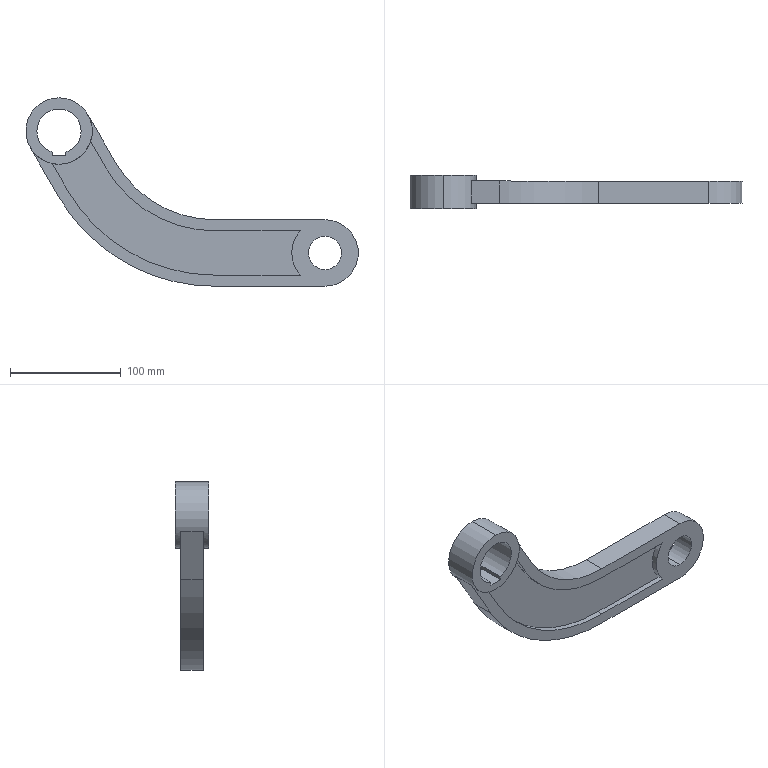Part | SolidWorks | features ICE 4, Extrusion 1 | 1 solid | 35 faces | box 300 x 30 x 170 mm | volume 285435 mm3 | plane 21 | cylinder 14 | commonest cylinder face diameters 60 x5 30 x2 226.795 x2 306.795 x2 40 x1 206.795 x1
STEP:
#1=CARTESIAN_POINT('',(240.,10.,-125.));
#2=VERTEX_POINT('',#1);
#3=CARTESIAN_POINT('',(240.,10.,-95.));
#4=VERTEX_POINT('',#3);
#5=CARTESIAN_POINT('',(240.,10.,-110.));
#6=DIRECTION('',(0.,1.,0.));
#7=DIRECTION('',(0.,0.,1.));
#8=AXIS2_PLACEMENT_3D('',#5,#6,#7);
#9=CIRCLE('',#8,15.);
#10=EDGE_CURVE('',#2,#4,#9,.T.);
#11=ORIENTED_EDGE('',*,*,#10,.T.);
#12=CARTESIAN_POINT('',(240.,-10.,-95.));
#13=VERTEX_POINT('',#12);
#14=CARTESIAN_POINT('',(240.,10.,-95.));
#15=DIRECTION('',(0.,-1.,0.));
#16=VECTOR('',#15,1000.);
#17=LINE('',#14,#16);
#18=EDGE_CURVE('',#4,#13,#17,.T.);
#19=ORIENTED_EDGE('',*,*,#18,.T.);
#20=CARTESIAN_POINT('',(240.,-10.,-125.));
#21=VERTEX_POINT('',#20);
#22=CARTESIAN_POINT('',(240.,-10.,-110.));
#23=DIRECTION('',(0.,1.,0.));
#24=DIRECTION('',(0.,0.,1.));
#25=AXIS2_PLACEMENT_3D('',#22,#23,#24);
#26=CIRCLE('',#25,15.);
#27=EDGE_CURVE('',#21,#13,#26,.T.);
#28=ORIENTED_EDGE('',*,*,#27,.F.);
#29=CARTESIAN_POINT('',(240.,10.,-125.));
#30=DIRECTION('',(0.,-1.,0.));
#31=VECTOR('',#30,1000.);
#32=LINE('',#29,#31);
#33=EDGE_CURVE('',#2,#21,#32,.T.);
#34=ORIENTED_EDGE('',*,*,#33,.F.);
#35=EDGE_LOOP('',(#11,#19,#28,#34));
#36=FACE_OUTER_BOUND('',#35,.T.);
#37=CARTESIAN_POINT('',(240.,10.,-110.));
#38=DIRECTION('',(0.,-1.,0.));
#39=DIRECTION('',(0.,0.,-1.));
#40=AXIS2_PLACEMENT_3D('',#37,#38,#39);
#41=CYLINDRICAL_SURFACE('',#40,15.);
#42=ADVANCED_FACE('',(#36),#41,.F.);
#43=CARTESIAN_POINT('',(0.,15.,30.));
#44=VERTEX_POINT('',#43);
#45=CARTESIAN_POINT('',(0.,15.,-30.));
#46=VERTEX_POINT('',#45);
#47=CARTESIAN_POINT('',(0.,15.,0.));
#48=DIRECTION('',(0.,1.,0.));
#49=DIRECTION('',(0.,0.,1.));
#50=AXIS2_PLACEMENT_3D('',#47,#48,#49);
#51=CIRCLE('',#50,30.);
#52=EDGE_CURVE('',#44,#46,#51,.T.);
#53=ORIENTED_EDGE('',*,*,#52,.F.);
#54=CARTESIAN_POINT('',(0.,-15.,30.));
#55=VERTEX_POINT('',#54);
#56=CARTESIAN_POINT('',(0.,15.,30.));
#57=DIRECTION('',(0.,-1.,0.));
#58=VECTOR('',#57,1000.);
#59=LINE('',#56,#58);
#60=EDGE_CURVE('',#44,#55,#59,.T.);
#61=ORIENTED_EDGE('',*,*,#60,.T.);
#62=CARTESIAN_POINT('',(0.,-15.,-30.));
#63=VERTEX_POINT('',#62);
#64=CARTESIAN_POINT('',(0.,-15.,0.));
#65=DIRECTION('',(0.,1.,0.));
#66=DIRECTION('',(0.,0.,1.));
#67=AXIS2_PLACEMENT_3D('',#64,#65,#66);
#68=CIRCLE('',#67,30.);
#69=EDGE_CURVE('',#55,#63,#68,.T.);
#70=ORIENTED_EDGE('',*,*,#69,.T.);
#71=CARTESIAN_POINT('',(0.,-5.,-30.));
#72=VERTEX_POINT('',#71);
#73=CARTESIAN_POINT('',(0.,15.,-30.));
#74=DIRECTION('',(0.,-1.,0.));
#75=VECTOR('',#74,1000.);
#76=LINE('',#73,#75);
#77=EDGE_CURVE('',#72,#63,#76,.T.);
#78=ORIENTED_EDGE('',*,*,#77,.F.);
#79=CARTESIAN_POINT('',(28.501,-5.,-9.365));
#80=VERTEX_POINT('',#79);
#81=CARTESIAN_POINT('',(0.,-5.,0.));
#82=DIRECTION('',(0.,1.,0.));
#83=DIRECTION('',(0.,0.,-1.));
#84=AXIS2_PLACEMENT_3D('',#81,#82,#83);
#85=CIRCLE('',#84,30.);
#86=EDGE_CURVE('',#80,#72,#85,.T.);
#87=ORIENTED_EDGE('',*,*,#86,.F.);
#88=CARTESIAN_POINT('',(28.501,-10.,-9.365));
#89=VERTEX_POINT('',#88);
#90=CARTESIAN_POINT('',(28.501,-5.,-9.365));
#91=DIRECTION('',(0.,-1.,0.));
#92=VECTOR('',#91,1000.);
#93=LINE('',#90,#92);
#94=EDGE_CURVE('',#80,#89,#93,.T.);
#95=ORIENTED_EDGE('',*,*,#94,.T.);
#96=CARTESIAN_POINT('',(25.981,-10.,15.));
#97=VERTEX_POINT('',#96);
#98=CARTESIAN_POINT('',(0.,-10.,0.));
#99=DIRECTION('',(0.,-1.,0.));
#100=DIRECTION('',(0.,0.,-1.));
#101=AXIS2_PLACEMENT_3D('',#98,#99,#100);
#102=CIRCLE('',#101,30.);
#103=EDGE_CURVE('',#89,#97,#102,.T.);
#104=ORIENTED_EDGE('',*,*,#103,.T.);
#105=CARTESIAN_POINT('',(25.981,10.,15.));
#106=VERTEX_POINT('',#105);
#107=CARTESIAN_POINT('',(25.981,10.,15.));
#108=DIRECTION('',(0.,-1.,0.));
#109=VECTOR('',#108,1000.);
#110=LINE('',#107,#109);
#111=EDGE_CURVE('',#106,#97,#110,.T.);
#112=ORIENTED_EDGE('',*,*,#111,.F.);
#113=CARTESIAN_POINT('',(28.501,10.,-9.365));
#114=VERTEX_POINT('',#113);
#115=CARTESIAN_POINT('',(0.,10.,0.));
#116=DIRECTION('',(0.,-1.,0.));
#117=DIRECTION('',(0.,0.,-1.));
#118=AXIS2_PLACEMENT_3D('',#115,#116,#117);
#119=CIRCLE('',#118,30.);
#120=EDGE_CURVE('',#114,#106,#119,.T.);
#121=ORIENTED_EDGE('',*,*,#120,.F.);
#122=CARTESIAN_POINT('',(28.501,5.,-9.365));
#123=VERTEX_POINT('',#122);
#124=CARTESIAN_POINT('',(28.501,5.,-9.365));
#125=DIRECTION('',(0.,1.,0.));
#126=VECTOR('',#125,1000.);
#127=LINE('',#124,#126);
#128=EDGE_CURVE('',#123,#114,#127,.T.);
#129=ORIENTED_EDGE('',*,*,#128,.F.);
#130=CARTESIAN_POINT('',(0.,5.,-30.));
#131=VERTEX_POINT('',#130);
#132=CARTESIAN_POINT('',(0.,5.,0.));
#133=DIRECTION('',(0.,-1.,0.));
#134=DIRECTION('',(0.,0.,1.));
#135=AXIS2_PLACEMENT_3D('',#132,#133,#134);
#136=CIRCLE('',#135,30.);
#137=EDGE_CURVE('',#131,#123,#136,.T.);
#138=ORIENTED_EDGE('',*,*,#137,.F.);
#139=CARTESIAN_POINT('',(0.,15.,-30.));
#140=DIRECTION('',(0.,-1.,0.));
#141=VECTOR('',#140,1000.);
#142=LINE('',#139,#141);
#143=EDGE_CURVE('',#46,#131,#142,.T.);
#144=ORIENTED_EDGE('',*,*,#143,.F.);
#145=EDGE_LOOP('',(#53,#61,#70,#78,#87,#95,#104,#112,#121,#129,#138,#144));
#146=FACE_OUTER_BOUND('',#145,.T.);
#147=CARTESIAN_POINT('',(0.,15.,0.));
#148=DIRECTION('',(0.,-1.,0.));
#149=DIRECTION('',(0.,0.,-1.));
#150=AXIS2_PLACEMENT_3D('',#147,#148,#149);
#151=CYLINDRICAL_SURFACE('',#150,30.);
#152=ADVANCED_FACE('',(#146),#151,.T.);
#153=ORIENTED_EDGE('',*,*,#60,.F.);
#154=CARTESIAN_POINT('',(0.,15.,0.));
#155=DIRECTION('',(0.,1.,0.));
#156=DIRECTION('',(0.,0.,1.));
#157=AXIS2_PLACEMENT_3D('',#154,#155,#156);
#158=CIRCLE('',#157,30.);
#159=EDGE_CURVE('',#46,#44,#158,.T.);
#160=ORIENTED_EDGE('',*,*,#159,.F.);
#161=ORIENTED_EDGE('',*,*,#143,.T.);
#162=CARTESIAN_POINT('',(-6.14,5.,-29.365));
#163=VERTEX_POINT('',#162);
#164=CARTESIAN_POINT('',(0.,5.,0.));
#165=DIRECTION('',(0.,-1.,0.));
#166=DIRECTION('',(0.,0.,1.));
#167=AXIS2_PLACEMENT_3D('',#164,#165,#166);
#168=CIRCLE('',#167,30.);
#169=EDGE_CURVE('',#163,#131,#168,.T.);
#170=ORIENTED_EDGE('',*,*,#169,.F.);
#171=CARTESIAN_POINT('',(-6.14,10.,-29.365));
#172=VERTEX_POINT('',#171);
#173=CARTESIAN_POINT('',(-6.14,5.,-29.365));
#174=DIRECTION('',(0.,1.,0.));
#175=VECTOR('',#174,1000.);
#176=LINE('',#173,#175);
#177=EDGE_CURVE('',#163,#172,#176,.T.);
#178=ORIENTED_EDGE('',*,*,#177,.T.);
#179=CARTESIAN_POINT('',(-25.981,10.,-15.));
#180=VERTEX_POINT('',#179);
#181=CARTESIAN_POINT('',(0.,10.,0.));
#182=DIRECTION('',(0.,-1.,0.));
#183=DIRECTION('',(0.,0.,-1.));
#184=AXIS2_PLACEMENT_3D('',#181,#182,#183);
#185=CIRCLE('',#184,30.);
#186=EDGE_CURVE('',#180,#172,#185,.T.);
#187=ORIENTED_EDGE('',*,*,#186,.F.);
#188=CARTESIAN_POINT('',(-25.981,-10.,-15.));
#189=VERTEX_POINT('',#188);
#190=CARTESIAN_POINT('',(-25.981,10.,-15.));
#191=DIRECTION('',(0.,-1.,0.));
#192=VECTOR('',#191,1000.);
#193=LINE('',#190,#192);
#194=EDGE_CURVE('',#180,#189,#193,.T.);
#195=ORIENTED_EDGE('',*,*,#194,.T.);
#196=CARTESIAN_POINT('',(-6.14,-10.,-29.365));
#197=VERTEX_POINT('',#196);
#198=CARTESIAN_POINT('',(0.,-10.,0.));
#199=DIRECTION('',(0.,-1.,0.));
#200=DIRECTION('',(0.,0.,-1.));
#201=AXIS2_PLACEMENT_3D('',#198,#199,#200);
#202=CIRCLE('',#201,30.);
#203=EDGE_CURVE('',#189,#197,#202,.T.);
#204=ORIENTED_EDGE('',*,*,#203,.T.);
#205=CARTESIAN_POINT('',(-6.14,-5.,-29.365));
#206=VERTEX_POINT('',#205);
#207=CARTESIAN_POINT('',(-6.14,-5.,-29.365));
#208=DIRECTION('',(0.,-1.,0.));
#209=VECTOR('',#208,1000.);
#210=LINE('',#207,#209);
#211=EDGE_CURVE('',#206,#197,#210,.T.);
#212=ORIENTED_EDGE('',*,*,#211,.F.);
#213=CARTESIAN_POINT('',(0.,-5.,0.));
#214=DIRECTION('',(0.,1.,0.));
#215=DIRECTION('',(0.,0.,-1.));
#216=AXIS2_PLACEMENT_3D('',#213,#214,#215);
#217=CIRCLE('',#216,30.);
#218=EDGE_CURVE('',#72,#206,#217,.T.);
#219=ORIENTED_EDGE('',*,*,#218,.F.);
#220=ORIENTED_EDGE('',*,*,#77,.T.);
#221=CARTESIAN_POINT('',(0.,-15.,0.));
#222=DIRECTION('',(0.,1.,0.));
#223=DIRECTION('',(0.,0.,1.));
#224=AXIS2_PLACEMENT_3D('',#221,#222,#223);
#225=CIRCLE('',#224,30.);
#226=EDGE_CURVE('',#63,#55,#225,.T.);
#227=ORIENTED_EDGE('',*,*,#226,.T.);
#228=EDGE_LOOP('',(#153,#160,#161,#170,#178,#187,#195,#204,#212,#219,#220,#227));
#229=FACE_OUTER_BOUND('',#228,.T.);
#230=CARTESIAN_POINT('',(0.,15.,0.));
#231=DIRECTION('',(0.,-1.,0.));
#232=DIRECTION('',(0.,0.,-1.));
#233=AXIS2_PLACEMENT_3D('',#230,#231,#232);
#234=CYLINDRICAL_SURFACE('',#233,30.);
#235=ADVANCED_FACE('',(#229),#234,.T.);
#236=ORIENTED_EDGE('',*,*,#159,.T.);
#237=ORIENTED_EDGE('',*,*,#52,.T.);
#238=EDGE_LOOP('',(#236,#237));
#239=FACE_OUTER_BOUND('',#238,.T.);
#240=CARTESIAN_POINT('',(-6.,15.,-22.379));
#241=VERTEX_POINT('',#240);
#242=CARTESIAN_POINT('',(-6.,15.,-19.079));
#243=VERTEX_POINT('',#242);
#244=CARTESIAN_POINT('',(-6.,15.,-22.379));
#245=DIRECTION('',(0.,0.,1.));
#246=VECTOR('',#245,1000.);
#247=LINE('',#244,#246);
#248=EDGE_CURVE('',#241,#243,#247,.T.);
#249=ORIENTED_EDGE('',*,*,#248,.F.);
#250=CARTESIAN_POINT('',(6.,15.,-22.379));
#251=VERTEX_POINT('',#250);
#252=CARTESIAN_POINT('',(6.,15.,-22.379));
#253=DIRECTION('',(-1.,0.,0.));
#254=VECTOR('',#253,1000.);
#255=LINE('',#252,#254);
#256=EDGE_CURVE('',#251,#241,#255,.T.);
#257=ORIENTED_EDGE('',*,*,#256,.F.);
#258=CARTESIAN_POINT('',(6.,15.,-19.079));
#259=VERTEX_POINT('',#258);
#260=CARTESIAN_POINT('',(6.,15.,-19.079));
#261=DIRECTION('',(0.,0.,-1.));
#262=VECTOR('',#261,1000.);
#263=LINE('',#260,#262);
#264=EDGE_CURVE('',#259,#251,#263,.T.);
#265=ORIENTED_EDGE('',*,*,#264,.F.);
#266=CARTESIAN_POINT('',(0.,15.,0.));
#267=DIRECTION('',(0.,1.,0.));
#268=DIRECTION('',(0.,0.,1.));
#269=AXIS2_PLACEMENT_3D('',#266,#267,#268);
#270=CIRCLE('',#269,20.);
#271=EDGE_CURVE('',#243,#259,#270,.T.);
#272=ORIENTED_EDGE('',*,*,#271,.F.);
#273=EDGE_LOOP('',(#249,#257,#265,#272));
#274=FACE_BOUND('',#273,.T.);
#275=CARTESIAN_POINT('',(0.,15.,0.));
#276=DIRECTION('',(0.,1.,0.));
#277=DIRECTION('',(0.,0.,1.));
#278=AXIS2_PLACEMENT_3D('',#275,#276,#277);
#279=PLANE('',#278);
#280=ADVANCED_FACE('',(#239,#274),#279,.T.);
#281=ORIENTED_EDGE('',*,*,#226,.F.);
#282=ORIENTED_EDGE('',*,*,#69,.F.);
#283=EDGE_LOOP('',(#281,#282));
#284=FACE_OUTER_BOUND('',#283,.T.);
#285=CARTESIAN_POINT('',(6.,-15.,-22.379));
#286=VERTEX_POINT('',#285);
#287=CARTESIAN_POINT('',(-6.,-15.,-22.379));
#288=VERTEX_POINT('',#287);
#289=CARTESIAN_POINT('',(6.,-15.,-22.379));
#290=DIRECTION('',(-1.,0.,0.));
#291=VECTOR('',#290,1000.);
#292=LINE('',#289,#291);
#293=EDGE_CURVE('',#286,#288,#292,.T.);
#294=ORIENTED_EDGE('',*,*,#293,.T.);
#295=CARTESIAN_POINT('',(-6.,-15.,-19.079));
#296=VERTEX_POINT('',#295);
#297=CARTESIAN_POINT('',(-6.,-15.,-22.379));
#298=DIRECTION('',(0.,0.,1.));
#299=VECTOR('',#298,1000.);
#300=LINE('',#297,#299);
#301=EDGE_CURVE('',#288,#296,#300,.T.);
#302=ORIENTED_EDGE('',*,*,#301,.T.);
#303=CARTESIAN_POINT('',(6.,-15.,-19.079));
#304=VERTEX_POINT('',#303);
#305=CARTESIAN_POINT('',(0.,-15.,0.));
#306=DIRECTION('',(0.,1.,0.));
#307=DIRECTION('',(0.,0.,1.));
#308=AXIS2_PLACEMENT_3D('',#305,#306,#307);
#309=CIRCLE('',#308,20.);
#310=EDGE_CURVE('',#296,#304,#309,.T.);
#311=ORIENTED_EDGE('',*,*,#310,.T.);
#312=CARTESIAN_POINT('',(6.,-15.,-19.079));
#313=DIRECTION('',(0.,0.,-1.));
#314=VECTOR('',#313,1000.);
#315=LINE('',#312,#314);
#316=EDGE_CURVE('',#304,#286,#315,.T.);
#317=ORIENTED_EDGE('',*,*,#316,.T.);
#318=EDGE_LOOP('',(#294,#302,#311,#317));
#319=FACE_BOUND('',#318,.T.);
#320=CARTESIAN_POINT('',(0.,-15.,0.));
#321=DIRECTION('',(0.,1.,0.));
#322=DIRECTION('',(0.,0.,1.));
#323=AXIS2_PLACEMENT_3D('',#320,#321,#322);
#324=PLANE('',#323);
#325=ADVANCED_FACE('',(#284,#319),#324,.F.);
#326=ORIENTED_EDGE('',*,*,#293,.F.);
#327=CARTESIAN_POINT('',(6.,15.,-22.379));
#328=DIRECTION('',(0.,-1.,0.));
#329=VECTOR('',#328,1000.);
#330=LINE('',#327,#329);
#331=EDGE_CURVE('',#251,#286,#330,.T.);
#332=ORIENTED_EDGE('',*,*,#331,.F.);
#333=ORIENTED_EDGE('',*,*,#256,.T.);
#334=CARTESIAN_POINT('',(-6.,15.,-22.379));
#335=DIRECTION('',(0.,-1.,0.));
#336=VECTOR('',#335,1000.);
#337=LINE('',#334,#336);
#338=EDGE_CURVE('',#241,#288,#337,.T.);
#339=ORIENTED_EDGE('',*,*,#338,.T.);
#340=EDGE_LOOP('',(#326,#332,#333,#339));
#341=FACE_OUTER_BOUND('',#340,.T.);
#342=CARTESIAN_POINT('',(6.,15.,-22.379));
#343=DIRECTION('',(0.,0.,1.));
#344=DIRECTION('',(1.,0.,0.));
#345=AXIS2_PLACEMENT_3D('',#342,#343,#344);
#346=PLANE('',#345);
#347=ADVANCED_FACE('',(#341),#346,.T.);
#348=ORIENTED_EDGE('',*,*,#301,.F.);
#349=ORIENTED_EDGE('',*,*,#338,.F.);
#350=ORIENTED_EDGE('',*,*,#248,.T.);
#351=CARTESIAN_POINT('',(-6.,15.,-19.079));
#352=DIRECTION('',(0.,-1.,0.));
#353=VECTOR('',#352,1000.);
#354=LINE('',#351,#353);
#355=EDGE_CURVE('',#243,#296,#354,.T.);
#356=ORIENTED_EDGE('',*,*,#355,.T.);
#357=EDGE_LOOP('',(#348,#349,#350,#356));
#358=FACE_OUTER_BOUND('',#357,.T.);
#359=CARTESIAN_POINT('',(-6.,15.,-22.379));
#360=DIRECTION('',(1.,0.,0.));
#361=DIRECTION('',(0.,0.,-1.));
#362=AXIS2_PLACEMENT_3D('',#359,#360,#361);
#363=PLANE('',#362);
#364=ADVANCED_FACE('',(#358),#363,.T.);
#365=ORIENTED_EDGE('',*,*,#310,.F.);
#366=ORIENTED_EDGE('',*,*,#355,.F.);
#367=ORIENTED_EDGE('',*,*,#271,.T.);
#368=CARTESIAN_POINT('',(6.,15.,-19.079));
#369=DIRECTION('',(0.,-1.,0.));
#370=VECTOR('',#369,1000.);
#371=LINE('',#368,#370);
#372=EDGE_CURVE('',#259,#304,#371,.T.);
#373=ORIENTED_EDGE('',*,*,#372,.T.);
#374=EDGE_LOOP('',(#365,#366,#367,#373));
#375=FACE_OUTER_BOUND('',#374,.T.);
#376=CARTESIAN_POINT('',(0.,15.,0.));
#377=DIRECTION('',(0.,-1.,0.));
#378=DIRECTION('',(0.,0.,-1.));
#379=AXIS2_PLACEMENT_3D('',#376,#377,#378);
#380=CYLINDRICAL_SURFACE('',#379,20.);
#381=ADVANCED_FACE('',(#375),#380,.F.);
#382=ORIENTED_EDGE('',*,*,#316,.F.);
#383=ORIENTED_EDGE('',*,*,#372,.F.);
#384=ORIENTED_EDGE('',*,*,#264,.T.);
#385=ORIENTED_EDGE('',*,*,#331,.T.);
#386=EDGE_LOOP('',(#382,#383,#384,#385));
#387=FACE_OUTER_BOUND('',#386,.T.);
#388=CARTESIAN_POINT('',(6.,15.,-19.079));
#389=DIRECTION('',(-1.,0.,0.));
#390=DIRECTION('',(0.,0.,1.));
#391=AXIS2_PLACEMENT_3D('',#388,#389,#390);
#392=PLANE('',#391);
#393=ADVANCED_FACE('',(#387),#392,.T.);
#394=CARTESIAN_POINT('',(42.321,10.,-33.301));
#395=VERTEX_POINT('',#394);
#396=CARTESIAN_POINT('',(140.526,10.,-90.));
#397=VERTEX_POINT('',#396);
#398=CARTESIAN_POINT('',(140.526,10.,23.397));
#399=DIRECTION('',(0.,-1.,0.));
#400=DIRECTION('',(0.,0.,1.));
#401=AXIS2_PLACEMENT_3D('',#398,#399,#400);
#402=CIRCLE('',#401,113.397);
#403=EDGE_CURVE('',#395,#397,#402,.T.);
#404=ORIENTED_EDGE('',*,*,#403,.F.);
#405=CARTESIAN_POINT('',(28.501,10.,-9.365));
#406=DIRECTION('',(0.5,0.,-0.866));
#407=VECTOR('',#406,1000.);
#408=LINE('',#405,#407);
#409=EDGE_CURVE('',#114,#395,#408,.T.);
#410=ORIENTED_EDGE('',*,*,#409,.F.);
#411=ORIENTED_EDGE('',*,*,#120,.T.);
#412=CARTESIAN_POINT('',(50.981,10.,-28.301));
#413=VERTEX_POINT('',#412);
#414=CARTESIAN_POINT('',(50.981,10.,-28.301));
#415=DIRECTION('',(0.5,0.,-0.866));
#416=VECTOR('',#415,1000.);
#417=LINE('',#414,#416);
#418=EDGE_CURVE('',#106,#413,#417,.T.);
#419=ORIENTED_EDGE('',*,*,#418,.T.);
#420=CARTESIAN_POINT('',(140.526,10.,-80.));
#421=VERTEX_POINT('',#420);
#422=CARTESIAN_POINT('',(140.526,10.,23.397));
#423=DIRECTION('',(0.,-1.,0.));
#424=DIRECTION('',(0.,0.,-1.));
#425=AXIS2_PLACEMENT_3D('',#422,#423,#424);
#426=CIRCLE('',#425,103.397);
#427=EDGE_CURVE('',#413,#421,#426,.T.);
#428=ORIENTED_EDGE('',*,*,#427,.T.);
#429=CARTESIAN_POINT('',(240.,10.,-80.));
#430=VERTEX_POINT('',#429);
#431=CARTESIAN_POINT('',(240.,10.,-80.));
#432=DIRECTION('',(1.,0.,0.));
#433=VECTOR('',#432,1000.);
#434=LINE('',#431,#433);
#435=EDGE_CURVE('',#421,#430,#434,.T.);
#436=ORIENTED_EDGE('',*,*,#435,.T.);
#437=CARTESIAN_POINT('',(240.,10.,-140.));
#438=VERTEX_POINT('',#437);
#439=CARTESIAN_POINT('',(240.,10.,-110.));
#440=DIRECTION('',(0.,1.,0.));
#441=DIRECTION('',(0.,0.,1.));
#442=AXIS2_PLACEMENT_3D('',#439,#440,#441);
#443=CIRCLE('',#442,30.);
#444=EDGE_CURVE('',#430,#438,#443,.T.);
#445=ORIENTED_EDGE('',*,*,#444,.T.);
#446=CARTESIAN_POINT('',(140.526,10.,-140.));
#447=VERTEX_POINT('',#446);
#448=CARTESIAN_POINT('',(140.526,10.,-140.));
#449=DIRECTION('',(-1.,0.,0.));
#450=VECTOR('',#449,1000.);
#451=LINE('',#448,#450);
#452=EDGE_CURVE('',#438,#447,#451,.T.);
#453=ORIENTED_EDGE('',*,*,#452,.T.);
#454=CARTESIAN_POINT('',(-0.9808,10.,-58.301));
#455=VERTEX_POINT('',#454);
#456=CARTESIAN_POINT('',(140.526,10.,23.397));
#457=DIRECTION('',(0.,1.,0.));
#458=DIRECTION('',(0.,0.,-1.));
#459=AXIS2_PLACEMENT_3D('',#456,#457,#458);
#460=CIRCLE('',#459,163.397);
#461=EDGE_CURVE('',#447,#455,#460,.T.);
#462=ORIENTED_EDGE('',*,*,#461,.T.);
#463=CARTESIAN_POINT('',(-25.981,10.,-15.));
#464=DIRECTION('',(-0.5,0.,0.866));
#465=VECTOR('',#464,1000.);
#466=LINE('',#463,#465);
#467=EDGE_CURVE('',#455,#180,#466,.T.);
#468=ORIENTED_EDGE('',*,*,#467,.T.);
#469=ORIENTED_EDGE('',*,*,#186,.T.);
#470=CARTESIAN_POINT('',(7.679,10.,-53.301));
#471=VERTEX_POINT('',#470);
#472=CARTESIAN_POINT('',(7.679,10.,-53.301));
#473=DIRECTION('',(-0.5,0.,0.866));
#474=VECTOR('',#473,1000.);
#475=LINE('',#472,#474);
#476=EDGE_CURVE('',#471,#172,#475,.T.);
#477=ORIENTED_EDGE('',*,*,#476,.F.);
#478=CARTESIAN_POINT('',(140.526,10.,-130.));
#479=VERTEX_POINT('',#478);
#480=CARTESIAN_POINT('',(140.526,10.,23.397));
#481=DIRECTION('',(0.,1.,0.));
#482=DIRECTION('',(0.,0.,1.));
#483=AXIS2_PLACEMENT_3D('',#480,#481,#482);
#484=CIRCLE('',#483,153.397);
#485=EDGE_CURVE('',#479,#471,#484,.T.);
#486=ORIENTED_EDGE('',*,*,#485,.F.);
#487=CARTESIAN_POINT('',(217.639,10.,-130.));
#488=VERTEX_POINT('',#487);
#489=CARTESIAN_POINT('',(217.639,10.,-130.));
#490=DIRECTION('',(-1.,0.,0.));
#491=VECTOR('',#490,1000.);
#492=LINE('',#489,#491);
#493=EDGE_CURVE('',#488,#479,#492,.T.);
#494=ORIENTED_EDGE('',*,*,#493,.F.);
#495=CARTESIAN_POINT('',(217.639,10.,-90.));
#496=VERTEX_POINT('',#495);
#497=CARTESIAN_POINT('',(240.,10.,-110.));
#498=DIRECTION('',(0.,-1.,0.));
#499=DIRECTION('',(0.,0.,1.));
#500=AXIS2_PLACEMENT_3D('',#497,#498,#499);
#501=CIRCLE('',#500,30.);
#502=EDGE_CURVE('',#496,#488,#501,.T.);
#503=ORIENTED_EDGE('',*,*,#502,.F.);
#504=CARTESIAN_POINT('',(140.526,10.,-90.));
#505=DIRECTION('',(1.,0.,0.));
#506=VECTOR('',#505,1000.);
#507=LINE('',#504,#506);
#508=EDGE_CURVE('',#397,#496,#507,.T.);
#509=ORIENTED_EDGE('',*,*,#508,.F.);
#510=EDGE_LOOP('',(#404,#410,#411,#419,#428,#436,#445,#453,#462,#468,#469,#477,#486,#494,#503,#509));
#511=FACE_OUTER_BOUND('',#510,.T.);
#512=ORIENTED_EDGE('',*,*,#10,.F.);
#513=CARTESIAN_POINT('',(240.,10.,-110.));
#514=DIRECTION('',(0.,1.,0.));
#515=DIRECTION('',(0.,0.,1.));
#516=AXIS2_PLACEMENT_3D('',#513,#514,#515);
#517=CIRCLE('',#516,15.);
#518=EDGE_CURVE('',#4,#2,#517,.T.);
#519=ORIENTED_EDGE('',*,*,#518,.F.);
#520=EDGE_LOOP('',(#512,#519));
#521=FACE_BOUND('',#520,.T.);
#522=CARTESIAN_POINT('',(0.,10.,0.));
#523=DIRECTION('',(0.,-1.,0.));
#524=DIRECTION('',(0.,0.,-1.));
#525=AXIS2_PLACEMENT_3D('',#522,#523,#524);
#526=PLANE('',#525);
#527=ADVANCED_FACE('',(#511,#521),#526,.F.);
#528=CARTESIAN_POINT('',(7.679,-10.,-53.301));
#529=VERTEX_POINT('',#528);
#530=CARTESIAN_POINT('',(-6.14,-10.,-29.365));
#531=DIRECTION('',(0.5,0.,-0.866));
#532=VECTOR('',#531,1000.);
#533=LINE('',#530,#532);
#534=EDGE_CURVE('',#197,#529,#533,.T.);
#535=ORIENTED_EDGE('',*,*,#534,.F.);
#536=ORIENTED_EDGE('',*,*,#203,.F.);
#537=CARTESIAN_POINT('',(-0.9808,-10.,-58.301));
#538=VERTEX_POINT('',#537);
#539=CARTESIAN_POINT('',(-25.981,-10.,-15.));
#540=DIRECTION('',(-0.5,0.,0.866));
#541=VECTOR('',#540,1000.);
#542=LINE('',#539,#541);
#543=EDGE_CURVE('',#538,#189,#542,.T.);
#544=ORIENTED_EDGE('',*,*,#543,.F.);
#545=CARTESIAN_POINT('',(140.526,-10.,-140.));
#546=VERTEX_POINT('',#545);
#547=CARTESIAN_POINT('',(140.526,-10.,23.397));
#548=DIRECTION('',(0.,1.,0.));
#549=DIRECTION('',(0.,0.,-1.));
#550=AXIS2_PLACEMENT_3D('',#547,#548,#549);
#551=CIRCLE('',#550,163.397);
#552=EDGE_CURVE('',#546,#538,#551,.T.);
#553=ORIENTED_EDGE('',*,*,#552,.F.);
#554=CARTESIAN_POINT('',(240.,-10.,-140.));
#555=VERTEX_POINT('',#554);
#556=CARTESIAN_POINT('',(140.526,-10.,-140.));
#557=DIRECTION('',(-1.,0.,0.));
#558=VECTOR('',#557,1000.);
#559=LINE('',#556,#558);
#560=EDGE_CURVE('',#555,#546,#559,.T.);
#561=ORIENTED_EDGE('',*,*,#560,.F.);
#562=CARTESIAN_POINT('',(240.,-10.,-80.));
#563=VERTEX_POINT('',#562);
#564=CARTESIAN_POINT('',(240.,-10.,-110.));
#565=DIRECTION('',(0.,1.,0.));
#566=DIRECTION('',(0.,0.,1.));
#567=AXIS2_PLACEMENT_3D('',#564,#565,#566);
#568=CIRCLE('',#567,30.);
#569=EDGE_CURVE('',#563,#555,#568,.T.);
#570=ORIENTED_EDGE('',*,*,#569,.F.);
#571=CARTESIAN_POINT('',(140.526,-10.,-80.));
#572=VERTEX_POINT('',#571);
#573=CARTESIAN_POINT('',(240.,-10.,-80.));
#574=DIRECTION('',(1.,0.,0.));
#575=VECTOR('',#574,1000.);
#576=LINE('',#573,#575);
#577=EDGE_CURVE('',#572,#563,#576,.T.);
#578=ORIENTED_EDGE('',*,*,#577,.F.);
#579=CARTESIAN_POINT('',(50.981,-10.,-28.301));
#580=VERTEX_POINT('',#579);
#581=CARTESIAN_POINT('',(140.526,-10.,23.397));
#582=DIRECTION('',(0.,-1.,0.));
#583=DIRECTION('',(0.,0.,-1.));
#584=AXIS2_PLACEMENT_3D('',#581,#582,#583);
#585=CIRCLE('',#584,103.397);
#586=EDGE_CURVE('',#580,#572,#585,.T.);
#587=ORIENTED_EDGE('',*,*,#586,.F.);
#588=CARTESIAN_POINT('',(50.981,-10.,-28.301));
#589=DIRECTION('',(0.5,0.,-0.866));
#590=VECTOR('',#589,1000.);
#591=LINE('',#588,#590);
#592=EDGE_CURVE('',#97,#580,#591,.T.);
#593=ORIENTED_EDGE('',*,*,#592,.F.);
#594=ORIENTED_EDGE('',*,*,#103,.F.);
#595=CARTESIAN_POINT('',(42.321,-10.,-33.301));
#596=VERTEX_POINT('',#595);
#597=CARTESIAN_POINT('',(28.501,-10.,-9.365));
#598=DIRECTION('',(-0.5,0.,0.866));
#599=VECTOR('',#598,1000.);
#600=LINE('',#597,#599);
#601=EDGE_CURVE('',#596,#89,#600,.T.);
#602=ORIENTED_EDGE('',*,*,#601,.F.);
#603=CARTESIAN_POINT('',(140.526,-10.,-90.));
#604=VERTEX_POINT('',#603);
#605=CARTESIAN_POINT('',(140.526,-10.,23.397));
#606=DIRECTION('',(0.,1.,0.));
#607=DIRECTION('',(0.,0.,1.));
#608=AXIS2_PLACEMENT_3D('',#605,#606,#607);
#609=CIRCLE('',#608,113.397);
#610=EDGE_CURVE('',#604,#596,#609,.T.);
#611=ORIENTED_EDGE('',*,*,#610,.F.);
#612=CARTESIAN_POINT('',(217.639,-10.,-90.));
#613=VERTEX_POINT('',#612);
#614=CARTESIAN_POINT('',(217.639,-10.,-90.));
#615=DIRECTION('',(-1.,0.,0.));
#616=VECTOR('',#615,1000.);
#617=LINE('',#614,#616);
#618=EDGE_CURVE('',#613,#604,#617,.T.);
#619=ORIENTED_EDGE('',*,*,#618,.F.);
#620=CARTESIAN_POINT('',(217.639,-10.,-130.));
#621=VERTEX_POINT('',#620);
#622=CARTESIAN_POINT('',(240.,-10.,-110.));
#623=DIRECTION('',(0.,1.,0.));
#624=DIRECTION('',(0.,0.,-1.));
#625=AXIS2_PLACEMENT_3D('',#622,#623,#624);
#626=CIRCLE('',#625,30.);
#627=EDGE_CURVE('',#621,#613,#626,.T.);
#628=ORIENTED_EDGE('',*,*,#627,.F.);
#629=CARTESIAN_POINT('',(140.526,-10.,-130.));
#630=VERTEX_POINT('',#629);
#631=CARTESIAN_POINT('',(217.639,-10.,-130.));
#632=DIRECTION('',(1.,0.,0.));
#633=VECTOR('',#632,1000.);
#634=LINE('',#631,#633);
#635=EDGE_CURVE('',#630,#621,#634,.T.);
#636=ORIENTED_EDGE('',*,*,#635,.F.);
#637=CARTESIAN_POINT('',(140.526,-10.,23.397));
#638=DIRECTION('',(0.,-1.,0.));
#639=DIRECTION('',(0.,0.,-1.));
#640=AXIS2_PLACEMENT_3D('',#637,#638,#639);
#641=CIRCLE('',#640,153.397);
#642=EDGE_CURVE('',#529,#630,#641,.T.);
#643=ORIENTED_EDGE('',*,*,#642,.F.);
#644=EDGE_LOOP('',(#535,#536,#544,#553,#561,#570,#578,#587,#593,#594,#602,#611,#619,#628,#636,#643));
#645=FACE_OUTER_BOUND('',#644,.T.);
#646=ORIENTED_EDGE('',*,*,#27,.T.);
#647=CARTESIAN_POINT('',(240.,-10.,-110.));
#648=DIRECTION('',(0.,1.,0.));
#649=DIRECTION('',(0.,0.,1.));
#650=AXIS2_PLACEMENT_3D('',#647,#648,#649);
#651=CIRCLE('',#650,15.);
#652=EDGE_CURVE('',#13,#21,#651,.T.);
#653=ORIENTED_EDGE('',*,*,#652,.T.);
#654=EDGE_LOOP('',(#646,#653));
#655=FACE_BOUND('',#654,.T.);
#656=CARTESIAN_POINT('',(0.,-10.,0.));
#657=DIRECTION('',(0.,-1.,0.));
#658=DIRECTION('',(0.,0.,-1.));
#659=AXIS2_PLACEMENT_3D('',#656,#657,#658);
#660=PLANE('',#659);
#661=ADVANCED_FACE('',(#645,#655),#660,.T.);
#662=ORIENTED_EDGE('',*,*,#592,.T.);
#663=CARTESIAN_POINT('',(50.981,10.,-28.301));
#664=DIRECTION('',(0.,-1.,0.));
#665=VECTOR('',#664,1000.);
#666=LINE('',#663,#665);
#667=EDGE_CURVE('',#413,#580,#666,.T.);
#668=ORIENTED_EDGE('',*,*,#667,.F.);
#669=ORIENTED_EDGE('',*,*,#418,.F.);
#670=ORIENTED_EDGE('',*,*,#111,.T.);
#671=EDGE_LOOP('',(#662,#668,#669,#670));
#672=FACE_OUTER_BOUND('',#671,.T.);
#673=CARTESIAN_POINT('',(50.981,10.,-28.301));
#674=DIRECTION('',(-0.866,0.,-0.5));
#675=DIRECTION('',(-0.5,0.,0.866));
#676=AXIS2_PLACEMENT_3D('',#673,#674,#675);
#677=PLANE('',#676);
#678=ADVANCED_FACE('',(#672),#677,.F.);
#679=ORIENTED_EDGE('',*,*,#586,.T.);
#680=CARTESIAN_POINT('',(140.526,10.,-80.));
#681=DIRECTION('',(0.,-1.,0.));
#682=VECTOR('',#681,1000.);
#683=LINE('',#680,#682);
#684=EDGE_CURVE('',#421,#572,#683,.T.);
#685=ORIENTED_EDGE('',*,*,#684,.F.);
#686=ORIENTED_EDGE('',*,*,#427,.F.);
#687=ORIENTED_EDGE('',*,*,#667,.T.);
#688=EDGE_LOOP('',(#679,#685,#686,#687));
#689=FACE_OUTER_BOUND('',#688,.T.);
#690=CARTESIAN_POINT('',(140.526,10.,23.397));
#691=DIRECTION('',(0.,-1.,0.));
#692=DIRECTION('',(0.,0.,-1.));
#693=AXIS2_PLACEMENT_3D('',#690,#691,#692);
#694=CYLINDRICAL_SURFACE('',#693,103.397);
#695=ADVANCED_FACE('',(#689),#694,.F.);
#696=ORIENTED_EDGE('',*,*,#577,.T.);
#697=CARTESIAN_POINT('',(240.,10.,-80.));
#698=DIRECTION('',(0.,-1.,0.));
#699=VECTOR('',#698,1000.);
#700=LINE('',#697,#699);
#701=EDGE_CURVE('',#430,#563,#700,.T.);
#702=ORIENTED_EDGE('',*,*,#701,.F.);
#703=ORIENTED_EDGE('',*,*,#435,.F.);
#704=ORIENTED_EDGE('',*,*,#684,.T.);
#705=EDGE_LOOP('',(#696,#702,#703,#704));
#706=FACE_OUTER_BOUND('',#705,.T.);
#707=CARTESIAN_POINT('',(240.,10.,-80.));
#708=DIRECTION('',(0.,0.,-1.));
#709=DIRECTION('',(-1.,0.,0.));
#710=AXIS2_PLACEMENT_3D('',#707,#708,#709);
#711=PLANE('',#710);
#712=ADVANCED_FACE('',(#706),#711,.F.);
#713=ORIENTED_EDGE('',*,*,#569,.T.);
#714=CARTESIAN_POINT('',(240.,10.,-140.));
#715=DIRECTION('',(0.,-1.,0.));
#716=VECTOR('',#715,1000.);
#717=LINE('',#714,#716);
#718=EDGE_CURVE('',#438,#555,#717,.T.);
#719=ORIENTED_EDGE('',*,*,#718,.F.);
#720=ORIENTED_EDGE('',*,*,#444,.F.);
#721=ORIENTED_EDGE('',*,*,#701,.T.);
#722=EDGE_LOOP('',(#713,#719,#720,#721));
#723=FACE_OUTER_BOUND('',#722,.T.);
#724=CARTESIAN_POINT('',(240.,10.,-110.));
#725=DIRECTION('',(0.,-1.,0.));
#726=DIRECTION('',(0.,0.,-1.));
#727=AXIS2_PLACEMENT_3D('',#724,#725,#726);
#728=CYLINDRICAL_SURFACE('',#727,30.);
#729=ADVANCED_FACE('',(#723),#728,.T.);
#730=ORIENTED_EDGE('',*,*,#560,.T.);
#731=CARTESIAN_POINT('',(140.526,10.,-140.));
#732=DIRECTION('',(0.,-1.,0.));
#733=VECTOR('',#732,1000.);
#734=LINE('',#731,#733);
#735=EDGE_CURVE('',#447,#546,#734,.T.);
#736=ORIENTED_EDGE('',*,*,#735,.F.);
#737=ORIENTED_EDGE('',*,*,#452,.F.);
#738=ORIENTED_EDGE('',*,*,#718,.T.);
#739=EDGE_LOOP('',(#730,#736,#737,#738));
#740=FACE_OUTER_BOUND('',#739,.T.);
#741=CARTESIAN_POINT('',(140.526,10.,-140.));
#742=DIRECTION('',(0.,0.,1.));
#743=DIRECTION('',(1.,0.,0.));
#744=AXIS2_PLACEMENT_3D('',#741,#742,#743);
#745=PLANE('',#744);
#746=ADVANCED_FACE('',(#740),#745,.F.);
#747=ORIENTED_EDGE('',*,*,#552,.T.);
#748=CARTESIAN_POINT('',(-0.9808,10.,-58.301));
#749=DIRECTION('',(0.,-1.,0.));
#750=VECTOR('',#749,1000.);
#751=LINE('',#748,#750);
#752=EDGE_CURVE('',#455,#538,#751,.T.);
#753=ORIENTED_EDGE('',*,*,#752,.F.);
#754=ORIENTED_EDGE('',*,*,#461,.F.);
#755=ORIENTED_EDGE('',*,*,#735,.T.);
#756=EDGE_LOOP('',(#747,#753,#754,#755));
#757=FACE_OUTER_BOUND('',#756,.T.);
#758=CARTESIAN_POINT('',(140.526,10.,23.397));
#759=DIRECTION('',(0.,-1.,0.));
#760=DIRECTION('',(0.,0.,-1.));
#761=AXIS2_PLACEMENT_3D('',#758,#759,#760);
#762=CYLINDRICAL_SURFACE('',#761,163.397);
#763=ADVANCED_FACE('',(#757),#762,.T.);
#764=ORIENTED_EDGE('',*,*,#543,.T.);
#765=ORIENTED_EDGE('',*,*,#194,.F.);
#766=ORIENTED_EDGE('',*,*,#467,.F.);
#767=ORIENTED_EDGE('',*,*,#752,.T.);
#768=EDGE_LOOP('',(#764,#765,#766,#767));
#769=FACE_OUTER_BOUND('',#768,.T.);
#770=CARTESIAN_POINT('',(-25.981,10.,-15.));
#771=DIRECTION('',(0.866,0.,0.5));
#772=DIRECTION('',(0.5,0.,-0.866));
#773=AXIS2_PLACEMENT_3D('',#770,#771,#772);
#774=PLANE('',#773);
#775=ADVANCED_FACE('',(#769),#774,.F.);
#776=ORIENTED_EDGE('',*,*,#18,.F.);
#777=ORIENTED_EDGE('',*,*,#518,.T.);
#778=ORIENTED_EDGE('',*,*,#33,.T.);
#779=ORIENTED_EDGE('',*,*,#652,.F.);
#780=EDGE_LOOP('',(#776,#777,#778,#779));
#781=FACE_OUTER_BOUND('',#780,.T.);
#782=CARTESIAN_POINT('',(240.,10.,-110.));
#783=DIRECTION('',(0.,-1.,0.));
#784=DIRECTION('',(0.,0.,-1.));
#785=AXIS2_PLACEMENT_3D('',#782,#783,#784);
#786=CYLINDRICAL_SURFACE('',#785,15.);
#787=ADVANCED_FACE('',(#781),#786,.F.);
#788=ORIENTED_EDGE('',*,*,#502,.T.);
#789=CARTESIAN_POINT('',(217.639,5.,-130.));
#790=VERTEX_POINT('',#789);
#791=CARTESIAN_POINT('',(217.639,5.,-130.));
#792=DIRECTION('',(0.,1.,0.));
#793=VECTOR('',#792,1000.);
#794=LINE('',#791,#793);
#795=EDGE_CURVE('',#790,#488,#794,.T.);
#796=ORIENTED_EDGE('',*,*,#795,.F.);
#797=CARTESIAN_POINT('',(217.639,5.,-90.));
#798=VERTEX_POINT('',#797);
#799=CARTESIAN_POINT('',(240.,5.,-110.));
#800=DIRECTION('',(0.,-1.,0.));
#801=DIRECTION('',(0.,0.,1.));
#802=AXIS2_PLACEMENT_3D('',#799,#800,#801);
#803=CIRCLE('',#802,30.);
#804=EDGE_CURVE('',#798,#790,#803,.T.);
#805=ORIENTED_EDGE('',*,*,#804,.F.);
#806=CARTESIAN_POINT('',(217.639,5.,-90.));
#807=DIRECTION('',(0.,1.,0.));
#808=VECTOR('',#807,1000.);
#809=LINE('',#806,#808);
#810=EDGE_CURVE('',#798,#496,#809,.T.);
#811=ORIENTED_EDGE('',*,*,#810,.T.);
#812=EDGE_LOOP('',(#788,#796,#805,#811));
#813=FACE_OUTER_BOUND('',#812,.T.);
#814=CARTESIAN_POINT('',(240.,5.,-110.));
#815=DIRECTION('',(0.,1.,0.));
#816=DIRECTION('',(0.,0.,1.));
#817=AXIS2_PLACEMENT_3D('',#814,#815,#816);
#818=CYLINDRICAL_SURFACE('',#817,30.);
#819=ADVANCED_FACE('',(#813),#818,.T.);
#820=ORIENTED_EDGE('',*,*,#508,.T.);
#821=ORIENTED_EDGE('',*,*,#810,.F.);
#822=CARTESIAN_POINT('',(140.526,5.,-90.));
#823=VERTEX_POINT('',#822);
#824=CARTESIAN_POINT('',(140.526,5.,-90.));
#825=DIRECTION('',(1.,0.,0.));
#826=VECTOR('',#825,1000.);
#827=LINE('',#824,#826);
#828=EDGE_CURVE('',#823,#798,#827,.T.);
#829=ORIENTED_EDGE('',*,*,#828,.F.);
#830=CARTESIAN_POINT('',(140.526,5.,-90.));
#831=DIRECTION('',(0.,1.,0.));
#832=VECTOR('',#831,1000.);
#833=LINE('',#830,#832);
#834=EDGE_CURVE('',#823,#397,#833,.T.);
#835=ORIENTED_EDGE('',*,*,#834,.T.);
#836=EDGE_LOOP('',(#820,#821,#829,#835));
#837=FACE_OUTER_BOUND('',#836,.T.);
#838=CARTESIAN_POINT('',(140.526,5.,-90.));
#839=DIRECTION('',(0.,0.,1.));
#840=DIRECTION('',(1.,0.,0.));
#841=AXIS2_PLACEMENT_3D('',#838,#839,#840);
#842=PLANE('',#841);
#843=ADVANCED_FACE('',(#837),#842,.F.);
#844=ORIENTED_EDGE('',*,*,#403,.T.);
#845=ORIENTED_EDGE('',*,*,#834,.F.);
#846=CARTESIAN_POINT('',(42.321,5.,-33.301));
#847=VERTEX_POINT('',#846);
#848=CARTESIAN_POINT('',(140.526,5.,23.397));
#849=DIRECTION('',(0.,-1.,0.));
#850=DIRECTION('',(0.,0.,1.));
#851=AXIS2_PLACEMENT_3D('',#848,#849,#850);
#852=CIRCLE('',#851,113.397);
#853=EDGE_CURVE('',#847,#823,#852,.T.);
#854=ORIENTED_EDGE('',*,*,#853,.F.);
#855=CARTESIAN_POINT('',(42.321,5.,-33.301));
#856=DIRECTION('',(0.,1.,0.));
#857=VECTOR('',#856,1000.);
#858=LINE('',#855,#857);
#859=EDGE_CURVE('',#847,#395,#858,.T.);
#860=ORIENTED_EDGE('',*,*,#859,.T.);
#861=EDGE_LOOP('',(#844,#845,#854,#860));
#862=FACE_OUTER_BOUND('',#861,.T.);
#863=CARTESIAN_POINT('',(140.526,5.,23.397));
#864=DIRECTION('',(0.,1.,0.));
#865=DIRECTION('',(0.,0.,1.));
#866=AXIS2_PLACEMENT_3D('',#863,#864,#865);
#867=CYLINDRICAL_SURFACE('',#866,113.397);
#868=ADVANCED_FACE('',(#862),#867,.T.);
#869=ORIENTED_EDGE('',*,*,#409,.T.);
#870=ORIENTED_EDGE('',*,*,#859,.F.);
#871=CARTESIAN_POINT('',(28.501,5.,-9.365));
#872=DIRECTION('',(0.5,0.,-0.866));
#873=VECTOR('',#872,1000.);
#874=LINE('',#871,#873);
#875=EDGE_CURVE('',#123,#847,#874,.T.);
#876=ORIENTED_EDGE('',*,*,#875,.F.);
#877=ORIENTED_EDGE('',*,*,#128,.T.);
#878=EDGE_LOOP('',(#869,#870,#876,#877));
#879=FACE_OUTER_BOUND('',#878,.T.);
#880=CARTESIAN_POINT('',(28.501,5.,-9.365));
#881=DIRECTION('',(0.866,0.,0.5));
#882=DIRECTION('',(0.5,0.,-0.866));
#883=AXIS2_PLACEMENT_3D('',#880,#881,#882);
#884=PLANE('',#883);
#885=ADVANCED_FACE('',(#879),#884,.F.);
#886=ORIENTED_EDGE('',*,*,#476,.T.);
#887=ORIENTED_EDGE('',*,*,#177,.F.);
#888=CARTESIAN_POINT('',(7.679,5.,-53.301));
#889=VERTEX_POINT('',#888);
#890=CARTESIAN_POINT('',(7.679,5.,-53.301));
#891=DIRECTION('',(-0.5,0.,0.866));
#892=VECTOR('',#891,1000.);
#893=LINE('',#890,#892);
#894=EDGE_CURVE('',#889,#163,#893,.T.);
#895=ORIENTED_EDGE('',*,*,#894,.F.);
#896=CARTESIAN_POINT('',(7.679,5.,-53.301));
#897=DIRECTION('',(0.,1.,0.));
#898=VECTOR('',#897,1000.);
#899=LINE('',#896,#898);
#900=EDGE_CURVE('',#889,#471,#899,.T.);
#901=ORIENTED_EDGE('',*,*,#900,.T.);
#902=EDGE_LOOP('',(#886,#887,#895,#901));
#903=FACE_OUTER_BOUND('',#902,.T.);
#904=CARTESIAN_POINT('',(7.679,5.,-53.301));
#905=DIRECTION('',(-0.866,0.,-0.5));
#906=DIRECTION('',(-0.5,0.,0.866));
#907=AXIS2_PLACEMENT_3D('',#904,#905,#906);
#908=PLANE('',#907);
#909=ADVANCED_FACE('',(#903),#908,.F.);
#910=ORIENTED_EDGE('',*,*,#485,.T.);
#911=ORIENTED_EDGE('',*,*,#900,.F.);
#912=CARTESIAN_POINT('',(140.526,5.,-130.));
#913=VERTEX_POINT('',#912);
#914=CARTESIAN_POINT('',(140.526,5.,23.397));
#915=DIRECTION('',(0.,1.,0.));
#916=DIRECTION('',(0.,0.,1.));
#917=AXIS2_PLACEMENT_3D('',#914,#915,#916);
#918=CIRCLE('',#917,153.397);
#919=EDGE_CURVE('',#913,#889,#918,.T.);
#920=ORIENTED_EDGE('',*,*,#919,.F.);
#921=CARTESIAN_POINT('',(140.526,5.,-130.));
#922=DIRECTION('',(0.,1.,0.));
#923=VECTOR('',#922,1000.);
#924=LINE('',#921,#923);
#925=EDGE_CURVE('',#913,#479,#924,.T.);
#926=ORIENTED_EDGE('',*,*,#925,.T.);
#927=EDGE_LOOP('',(#910,#911,#920,#926));
#928=FACE_OUTER_BOUND('',#927,.T.);
#929=CARTESIAN_POINT('',(140.526,5.,23.397));
#930=DIRECTION('',(0.,1.,0.));
#931=DIRECTION('',(0.,0.,1.));
#932=AXIS2_PLACEMENT_3D('',#929,#930,#931);
#933=CYLINDRICAL_SURFACE('',#932,153.397);
#934=ADVANCED_FACE('',(#928),#933,.F.);
#935=ORIENTED_EDGE('',*,*,#493,.T.);
#936=ORIENTED_EDGE('',*,*,#925,.F.);
#937=CARTESIAN_POINT('',(217.639,5.,-130.));
#938=DIRECTION('',(-1.,0.,0.));
#939=VECTOR('',#938,1000.);
#940=LINE('',#937,#939);
#941=EDGE_CURVE('',#790,#913,#940,.T.);
#942=ORIENTED_EDGE('',*,*,#941,.F.);
#943=ORIENTED_EDGE('',*,*,#795,.T.);
#944=EDGE_LOOP('',(#935,#936,#942,#943));
#945=FACE_OUTER_BOUND('',#944,.T.);
#946=CARTESIAN_POINT('',(217.639,5.,-130.));
#947=DIRECTION('',(0.,0.,-1.));
#948=DIRECTION('',(-1.,0.,0.));
#949=AXIS2_PLACEMENT_3D('',#946,#947,#948);
#950=PLANE('',#949);
#951=ADVANCED_FACE('',(#945),#950,.F.);
#952=ORIENTED_EDGE('',*,*,#804,.T.);
#953=ORIENTED_EDGE('',*,*,#941,.T.);
#954=ORIENTED_EDGE('',*,*,#919,.T.);
#955=ORIENTED_EDGE('',*,*,#894,.T.);
#956=ORIENTED_EDGE('',*,*,#169,.T.);
#957=ORIENTED_EDGE('',*,*,#137,.T.);
#958=ORIENTED_EDGE('',*,*,#875,.T.);
#959=ORIENTED_EDGE('',*,*,#853,.T.);
#960=ORIENTED_EDGE('',*,*,#828,.T.);
#961=EDGE_LOOP('',(#952,#953,#954,#955,#956,#957,#958,#959,#960));
#962=FACE_OUTER_BOUND('',#961,.T.);
#963=CARTESIAN_POINT('',(240.,5.,-110.));
#964=DIRECTION('',(0.,1.,0.));
#965=DIRECTION('',(0.,0.,1.));
#966=AXIS2_PLACEMENT_3D('',#963,#964,#965);
#967=PLANE('',#966);
#968=ADVANCED_FACE('',(#962),#967,.T.);
#969=ORIENTED_EDGE('',*,*,#627,.T.);
#970=CARTESIAN_POINT('',(217.639,-5.,-90.));
#971=VERTEX_POINT('',#970);
#972=CARTESIAN_POINT('',(217.639,-5.,-90.));
#973=DIRECTION('',(0.,-1.,0.));
#974=VECTOR('',#973,1000.);
#975=LINE('',#972,#974);
#976=EDGE_CURVE('',#971,#613,#975,.T.);
#977=ORIENTED_EDGE('',*,*,#976,.F.);
#978=CARTESIAN_POINT('',(217.639,-5.,-130.));
#979=VERTEX_POINT('',#978);
#980=CARTESIAN_POINT('',(240.,-5.,-110.));
#981=DIRECTION('',(0.,1.,0.));
#982=DIRECTION('',(0.,0.,-1.));
#983=AXIS2_PLACEMENT_3D('',#980,#981,#982);
#984=CIRCLE('',#983,30.);
#985=EDGE_CURVE('',#979,#971,#984,.T.);
#986=ORIENTED_EDGE('',*,*,#985,.F.);
#987=CARTESIAN_POINT('',(217.639,-5.,-130.));
#988=DIRECTION('',(0.,-1.,0.));
#989=VECTOR('',#988,1000.);
#990=LINE('',#987,#989);
#991=EDGE_CURVE('',#979,#621,#990,.T.);
#992=ORIENTED_EDGE('',*,*,#991,.T.);
#993=EDGE_LOOP('',(#969,#977,#986,#992));
#994=FACE_OUTER_BOUND('',#993,.T.);
#995=CARTESIAN_POINT('',(240.,-5.,-110.));
#996=DIRECTION('',(0.,-1.,0.));
#997=DIRECTION('',(0.,0.,-1.));
#998=AXIS2_PLACEMENT_3D('',#995,#996,#997);
#999=CYLINDRICAL_SURFACE('',#998,30.);
#1000=ADVANCED_FACE('',(#994),#999,.T.);
#1001=ORIENTED_EDGE('',*,*,#635,.T.);
#1002=ORIENTED_EDGE('',*,*,#991,.F.);
#1003=CARTESIAN_POINT('',(140.526,-5.,-130.));
#1004=VERTEX_POINT('',#1003);
#1005=CARTESIAN_POINT('',(217.639,-5.,-130.));
#1006=DIRECTION('',(1.,0.,0.));
#1007=VECTOR('',#1006,1000.);
#1008=LINE('',#1005,#1007);
#1009=EDGE_CURVE('',#1004,#979,#1008,.T.);
#1010=ORIENTED_EDGE('',*,*,#1009,.F.);
#1011=CARTESIAN_POINT('',(140.526,-5.,-130.));
#1012=DIRECTION('',(0.,-1.,0.));
#1013=VECTOR('',#1012,1000.);
#1014=LINE('',#1011,#1013);
#1015=EDGE_CURVE('',#1004,#630,#1014,.T.);
#1016=ORIENTED_EDGE('',*,*,#1015,.T.);
#1017=EDGE_LOOP('',(#1001,#1002,#1010,#1016));
#1018=FACE_OUTER_BOUND('',#1017,.T.);
#1019=CARTESIAN_POINT('',(217.639,-5.,-130.));
#1020=DIRECTION('',(0.,0.,-1.));
#1021=DIRECTION('',(-1.,0.,0.));
#1022=AXIS2_PLACEMENT_3D('',#1019,#1020,#1021);
#1023=PLANE('',#1022);
#1024=ADVANCED_FACE('',(#1018),#1023,.F.);
#1025=ORIENTED_EDGE('',*,*,#642,.T.);
#1026=ORIENTED_EDGE('',*,*,#1015,.F.);
#1027=CARTESIAN_POINT('',(7.679,-5.,-53.301));
#1028=VERTEX_POINT('',#1027);
#1029=CARTESIAN_POINT('',(140.526,-5.,23.397));
#1030=DIRECTION('',(0.,-1.,0.));
#1031=DIRECTION('',(0.,0.,-1.));
#1032=AXIS2_PLACEMENT_3D('',#1029,#1030,#1031);
#1033=CIRCLE('',#1032,153.397);
#1034=EDGE_CURVE('',#1028,#1004,#1033,.T.);
#1035=ORIENTED_EDGE('',*,*,#1034,.F.);
#1036=CARTESIAN_POINT('',(7.679,-5.,-53.301));
#1037=DIRECTION('',(0.,-1.,0.));
#1038=VECTOR('',#1037,1000.);
#1039=LINE('',#1036,#1038);
#1040=EDGE_CURVE('',#1028,#529,#1039,.T.);
#1041=ORIENTED_EDGE('',*,*,#1040,.T.);
#1042=EDGE_LOOP('',(#1025,#1026,#1035,#1041));
#1043=FACE_OUTER_BOUND('',#1042,.T.);
#1044=CARTESIAN_POINT('',(140.526,-5.,23.397));
#1045=DIRECTION('',(0.,-1.,0.));
#1046=DIRECTION('',(0.,0.,-1.));
#1047=AXIS2_PLACEMENT_3D('',#1044,#1045,#1046);
#1048=CYLINDRICAL_SURFACE('',#1047,153.397);
#1049=ADVANCED_FACE('',(#1043),#1048,.F.);
#1050=ORIENTED_EDGE('',*,*,#534,.T.);
#1051=ORIENTED_EDGE('',*,*,#1040,.F.);
#1052=CARTESIAN_POINT('',(-6.14,-5.,-29.365));
#1053=DIRECTION('',(0.5,0.,-0.866));
#1054=VECTOR('',#1053,1000.);
#1055=LINE('',#1052,#1054);
#1056=EDGE_CURVE('',#206,#1028,#1055,.T.);
#1057=ORIENTED_EDGE('',*,*,#1056,.F.);
#1058=ORIENTED_EDGE('',*,*,#211,.T.);
#1059=EDGE_LOOP('',(#1050,#1051,#1057,#1058));
#1060=FACE_OUTER_BOUND('',#1059,.T.);
#1061=CARTESIAN_POINT('',(-6.14,-5.,-29.365));
#1062=DIRECTION('',(-0.866,0.,-0.5));
#1063=DIRECTION('',(-0.5,0.,0.866));
#1064=AXIS2_PLACEMENT_3D('',#1061,#1062,#1063);
#1065=PLANE('',#1064);
#1066=ADVANCED_FACE('',(#1060),#1065,.F.);
#1067=ORIENTED_EDGE('',*,*,#601,.T.);
#1068=ORIENTED_EDGE('',*,*,#94,.F.);
#1069=CARTESIAN_POINT('',(42.321,-5.,-33.301));
#1070=VERTEX_POINT('',#1069);
#1071=CARTESIAN_POINT('',(28.501,-5.,-9.365));
#1072=DIRECTION('',(-0.5,0.,0.866));
#1073=VECTOR('',#1072,1000.);
#1074=LINE('',#1071,#1073);
#1075=EDGE_CURVE('',#1070,#80,#1074,.T.);
#1076=ORIENTED_EDGE('',*,*,#1075,.F.);
#1077=CARTESIAN_POINT('',(42.321,-5.,-33.301));
#1078=DIRECTION('',(0.,-1.,0.));
#1079=VECTOR('',#1078,1000.);
#1080=LINE('',#1077,#1079);
#1081=EDGE_CURVE('',#1070,#596,#1080,.T.);
#1082=ORIENTED_EDGE('',*,*,#1081,.T.);
#1083=EDGE_LOOP('',(#1067,#1068,#1076,#1082));
#1084=FACE_OUTER_BOUND('',#1083,.T.);
#1085=CARTESIAN_POINT('',(28.501,-5.,-9.365));
#1086=DIRECTION('',(0.866,0.,0.5));
#1087=DIRECTION('',(0.5,0.,-0.866));
#1088=AXIS2_PLACEMENT_3D('',#1085,#1086,#1087);
#1089=PLANE('',#1088);
#1090=ADVANCED_FACE('',(#1084),#1089,.F.);
#1091=ORIENTED_EDGE('',*,*,#610,.T.);
#1092=ORIENTED_EDGE('',*,*,#1081,.F.);
#1093=CARTESIAN_POINT('',(140.526,-5.,-90.));
#1094=VERTEX_POINT('',#1093);
#1095=CARTESIAN_POINT('',(140.526,-5.,23.397));
#1096=DIRECTION('',(0.,1.,0.));
#1097=DIRECTION('',(0.,0.,1.));
#1098=AXIS2_PLACEMENT_3D('',#1095,#1096,#1097);
#1099=CIRCLE('',#1098,113.397);
#1100=EDGE_CURVE('',#1094,#1070,#1099,.T.);
#1101=ORIENTED_EDGE('',*,*,#1100,.F.);
#1102=CARTESIAN_POINT('',(140.526,-5.,-90.));
#1103=DIRECTION('',(0.,-1.,0.));
#1104=VECTOR('',#1103,1000.);
#1105=LINE('',#1102,#1104);
#1106=EDGE_CURVE('',#1094,#604,#1105,.T.);
#1107=ORIENTED_EDGE('',*,*,#1106,.T.);
#1108=EDGE_LOOP('',(#1091,#1092,#1101,#1107));
#1109=FACE_OUTER_BOUND('',#1108,.T.);
#1110=CARTESIAN_POINT('',(140.526,-5.,23.397));
#1111=DIRECTION('',(0.,-1.,0.));
#1112=DIRECTION('',(0.,0.,-1.));
#1113=AXIS2_PLACEMENT_3D('',#1110,#1111,#1112);
#1114=CYLINDRICAL_SURFACE('',#1113,113.397);
#1115=ADVANCED_FACE('',(#1109),#1114,.T.);
#1116=ORIENTED_EDGE('',*,*,#618,.T.);
#1117=ORIENTED_EDGE('',*,*,#1106,.F.);
#1118=CARTESIAN_POINT('',(217.639,-5.,-90.));
#1119=DIRECTION('',(-1.,0.,0.));
#1120=VECTOR('',#1119,1000.);
#1121=LINE('',#1118,#1120);
#1122=EDGE_CURVE('',#971,#1094,#1121,.T.);
#1123=ORIENTED_EDGE('',*,*,#1122,.F.);
#1124=ORIENTED_EDGE('',*,*,#976,.T.);
#1125=EDGE_LOOP('',(#1116,#1117,#1123,#1124));
#1126=FACE_OUTER_BOUND('',#1125,.T.);
#1127=CARTESIAN_POINT('',(217.639,-5.,-90.));
#1128=DIRECTION('',(0.,0.,1.));
#1129=DIRECTION('',(1.,0.,0.));
#1130=AXIS2_PLACEMENT_3D('',#1127,#1128,#1129);
#1131=PLANE('',#1130);
#1132=ADVANCED_FACE('',(#1126),#1131,.F.);
#1133=ORIENTED_EDGE('',*,*,#985,.T.);
#1134=ORIENTED_EDGE('',*,*,#1122,.T.);
#1135=ORIENTED_EDGE('',*,*,#1100,.T.);
#1136=ORIENTED_EDGE('',*,*,#1075,.T.);
#1137=ORIENTED_EDGE('',*,*,#86,.T.);
#1138=ORIENTED_EDGE('',*,*,#218,.T.);
#1139=ORIENTED_EDGE('',*,*,#1056,.T.);
#1140=ORIENTED_EDGE('',*,*,#1034,.T.);
#1141=ORIENTED_EDGE('',*,*,#1009,.T.);
#1142=EDGE_LOOP('',(#1133,#1134,#1135,#1136,#1137,#1138,#1139,#1140,#1141));
#1143=FACE_OUTER_BOUND('',#1142,.T.);
#1144=CARTESIAN_POINT('',(240.,-5.,-110.));
#1145=DIRECTION('',(0.,-1.,0.));
#1146=DIRECTION('',(0.,0.,-1.));
#1147=AXIS2_PLACEMENT_3D('',#1144,#1145,#1146);
#1148=PLANE('',#1147);
#1149=ADVANCED_FACE('',(#1143),#1148,.T.);
#1150=CLOSED_SHELL('',(#42,#152,#235,#280,#325,#347,#364,#381,#393,#527,#661,#678,#695,#712,#729,#746,#763,#775,#787,#819,#843,#868,#885,#909,#934,#951,#968,#1000,#1024,#1049,#1066,#1090,#1115,#1132,#1149));
#1151=MANIFOLD_SOLID_BREP('',#1150);
#1152=CARTESIAN_POINT('',(0.,0.,0.));
#1153=DIRECTION('',(0.,0.,1.));
#1154=DIRECTION('',(1.,0.,0.));
#1155=AXIS2_PLACEMENT_3D('',#1152,#1153,#1154);
#1156=(LENGTH_UNIT()NAMED_UNIT(*)SI_UNIT(.MILLI.,.METRE.));
#1157=UNCERTAINTY_MEASURE_WITH_UNIT(LENGTH_MEASURE(0.00001),#1156,'','');
#1158=(NAMED_UNIT(*)PLANE_ANGLE_UNIT()SI_UNIT($,.RADIAN.));
#1159=(NAMED_UNIT(*)SI_UNIT($,.STERADIAN.)SOLID_ANGLE_UNIT());
#1160=(GEOMETRIC_REPRESENTATION_CONTEXT(3)GLOBAL_UNCERTAINTY_ASSIGNED_CONTEXT((#1157))GLOBAL_UNIT_ASSIGNED_CONTEXT((#1156,#1158,#1159))REPRESENTATION_CONTEXT('',''));
#1161=ADVANCED_BREP_SHAPE_REPRESENTATION('',(#1151,#1155),#1160);